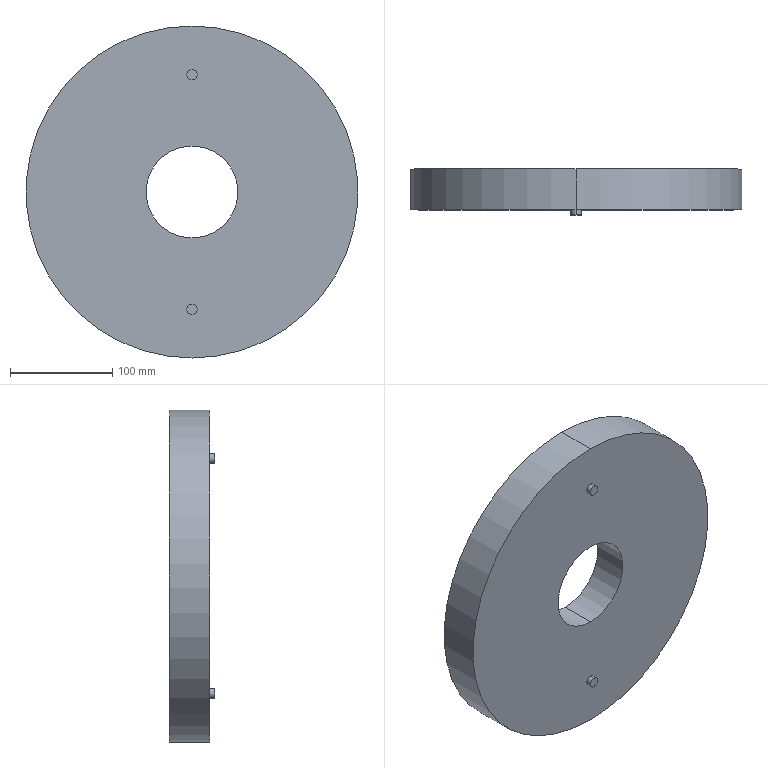Part | SolidWorks | features BaseBody 1 | 1 solid | 15 faces | box 325 x 45 x 325 mm | volume 2743003 mm3 | cylinder 10 | plane 5 | commonest cylinder face diameters 10 x4 90 x2 300 x2 325 x2
STEP:
#1=CARTESIAN_POINT('',(0.,-5.,110.));
#2=VERTEX_POINT('',#1);
#3=CARTESIAN_POINT('',(0.,-5.,120.));
#4=VERTEX_POINT('',#3);
#5=CARTESIAN_POINT('',(0.,-5.,115.));
#6=DIRECTION('',(0.,-1.,0.));
#7=DIRECTION('',(0.,0.,-1.));
#8=AXIS2_PLACEMENT_3D('',#5,#6,#7);
#9=CIRCLE('',#8,5.);
#10=EDGE_CURVE('',#2,#4,#9,.T.);
#11=ORIENTED_EDGE('',*,*,#10,.F.);
#12=CARTESIAN_POINT('',(0.,0.,110.));
#13=VERTEX_POINT('',#12);
#14=CARTESIAN_POINT('',(0.,-5.,110.));
#15=DIRECTION('',(0.,1.,0.));
#16=VECTOR('',#15,1000.);
#17=LINE('',#14,#16);
#18=EDGE_CURVE('',#2,#13,#17,.T.);
#19=ORIENTED_EDGE('',*,*,#18,.T.);
#20=CARTESIAN_POINT('',(0.,0.,120.));
#21=VERTEX_POINT('',#20);
#22=CARTESIAN_POINT('',(0.,0.,115.));
#23=DIRECTION('',(0.,-1.,0.));
#24=DIRECTION('',(0.,0.,1.));
#25=AXIS2_PLACEMENT_3D('',#22,#23,#24);
#26=CIRCLE('',#25,5.);
#27=EDGE_CURVE('',#13,#21,#26,.T.);
#28=ORIENTED_EDGE('',*,*,#27,.T.);
#29=CARTESIAN_POINT('',(0.,-5.,120.));
#30=DIRECTION('',(0.,1.,0.));
#31=VECTOR('',#30,1000.);
#32=LINE('',#29,#31);
#33=EDGE_CURVE('',#4,#21,#32,.T.);
#34=ORIENTED_EDGE('',*,*,#33,.F.);
#35=EDGE_LOOP('',(#11,#19,#28,#34));
#36=FACE_OUTER_BOUND('',#35,.T.);
#37=CARTESIAN_POINT('',(0.,-5.,115.));
#38=DIRECTION('',(0.,1.,0.));
#39=DIRECTION('',(0.,0.,1.));
#40=AXIS2_PLACEMENT_3D('',#37,#38,#39);
#41=CYLINDRICAL_SURFACE('',#40,5.);
#42=ADVANCED_FACE('',(#36),#41,.T.);
#43=CARTESIAN_POINT('',(0.,-5.,-120.));
#44=VERTEX_POINT('',#43);
#45=CARTESIAN_POINT('',(0.,-5.,-110.));
#46=VERTEX_POINT('',#45);
#47=CARTESIAN_POINT('',(0.,-5.,-115.));
#48=DIRECTION('',(0.,-1.,0.));
#49=DIRECTION('',(0.,0.,-1.));
#50=AXIS2_PLACEMENT_3D('',#47,#48,#49);
#51=CIRCLE('',#50,5.);
#52=EDGE_CURVE('',#44,#46,#51,.T.);
#53=ORIENTED_EDGE('',*,*,#52,.F.);
#54=CARTESIAN_POINT('',(0.,0.,-120.));
#55=VERTEX_POINT('',#54);
#56=CARTESIAN_POINT('',(0.,-5.,-120.));
#57=DIRECTION('',(0.,1.,0.));
#58=VECTOR('',#57,1000.);
#59=LINE('',#56,#58);
#60=EDGE_CURVE('',#44,#55,#59,.T.);
#61=ORIENTED_EDGE('',*,*,#60,.T.);
#62=CARTESIAN_POINT('',(0.,0.,-110.));
#63=VERTEX_POINT('',#62);
#64=CARTESIAN_POINT('',(0.,0.,-115.));
#65=DIRECTION('',(0.,-1.,0.));
#66=DIRECTION('',(0.,0.,1.));
#67=AXIS2_PLACEMENT_3D('',#64,#65,#66);
#68=CIRCLE('',#67,5.);
#69=EDGE_CURVE('',#55,#63,#68,.T.);
#70=ORIENTED_EDGE('',*,*,#69,.T.);
#71=CARTESIAN_POINT('',(0.,-5.,-110.));
#72=DIRECTION('',(0.,1.,0.));
#73=VECTOR('',#72,1000.);
#74=LINE('',#71,#73);
#75=EDGE_CURVE('',#46,#63,#74,.T.);
#76=ORIENTED_EDGE('',*,*,#75,.F.);
#77=EDGE_LOOP('',(#53,#61,#70,#76));
#78=FACE_OUTER_BOUND('',#77,.T.);
#79=CARTESIAN_POINT('',(0.,-5.,-115.));
#80=DIRECTION('',(0.,1.,0.));
#81=DIRECTION('',(0.,0.,1.));
#82=AXIS2_PLACEMENT_3D('',#79,#80,#81);
#83=CYLINDRICAL_SURFACE('',#82,5.);
#84=ADVANCED_FACE('',(#78),#83,.T.);
#85=CARTESIAN_POINT('',(0.,0.,-45.));
#86=VERTEX_POINT('',#85);
#87=CARTESIAN_POINT('',(0.,0.,45.));
#88=VERTEX_POINT('',#87);
#89=CARTESIAN_POINT('',(0.,0.,0.));
#90=DIRECTION('',(0.,1.,0.));
#91=DIRECTION('',(0.,0.,1.));
#92=AXIS2_PLACEMENT_3D('',#89,#90,#91);
#93=CIRCLE('',#92,45.);
#94=EDGE_CURVE('',#86,#88,#93,.T.);
#95=ORIENTED_EDGE('',*,*,#94,.F.);
#96=CARTESIAN_POINT('',(0.,35.,-45.));
#97=VERTEX_POINT('',#96);
#98=CARTESIAN_POINT('',(0.,0.,-45.));
#99=DIRECTION('',(0.,1.,0.));
#100=VECTOR('',#99,1000.);
#101=LINE('',#98,#100);
#102=EDGE_CURVE('',#86,#97,#101,.T.);
#103=ORIENTED_EDGE('',*,*,#102,.T.);
#104=CARTESIAN_POINT('',(0.,35.,45.));
#105=VERTEX_POINT('',#104);
#106=CARTESIAN_POINT('',(0.,35.,0.));
#107=DIRECTION('',(0.,1.,0.));
#108=DIRECTION('',(0.,0.,1.));
#109=AXIS2_PLACEMENT_3D('',#106,#107,#108);
#110=CIRCLE('',#109,45.);
#111=EDGE_CURVE('',#97,#105,#110,.T.);
#112=ORIENTED_EDGE('',*,*,#111,.T.);
#113=CARTESIAN_POINT('',(0.,0.,45.));
#114=DIRECTION('',(0.,1.,0.));
#115=VECTOR('',#114,1000.);
#116=LINE('',#113,#115);
#117=EDGE_CURVE('',#88,#105,#116,.T.);
#118=ORIENTED_EDGE('',*,*,#117,.F.);
#119=EDGE_LOOP('',(#95,#103,#112,#118));
#120=FACE_OUTER_BOUND('',#119,.T.);
#121=CARTESIAN_POINT('',(0.,0.,0.));
#122=DIRECTION('',(0.,1.,0.));
#123=DIRECTION('',(0.,0.,1.));
#124=AXIS2_PLACEMENT_3D('',#121,#122,#123);
#125=CYLINDRICAL_SURFACE('',#124,45.);
#126=ADVANCED_FACE('',(#120),#125,.F.);
#127=CARTESIAN_POINT('',(0.,35.,-150.));
#128=VERTEX_POINT('',#127);
#129=CARTESIAN_POINT('',(0.,35.,150.));
#130=VERTEX_POINT('',#129);
#131=CARTESIAN_POINT('',(0.,35.,0.));
#132=DIRECTION('',(0.,1.,0.));
#133=DIRECTION('',(0.,0.,1.));
#134=AXIS2_PLACEMENT_3D('',#131,#132,#133);
#135=CIRCLE('',#134,150.);
#136=EDGE_CURVE('',#128,#130,#135,.T.);
#137=ORIENTED_EDGE('',*,*,#136,.F.);
#138=CARTESIAN_POINT('',(0.,40.,-150.));
#139=VERTEX_POINT('',#138);
#140=CARTESIAN_POINT('',(0.,35.,-150.));
#141=DIRECTION('',(0.,1.,0.));
#142=VECTOR('',#141,1000.);
#143=LINE('',#140,#142);
#144=EDGE_CURVE('',#128,#139,#143,.T.);
#145=ORIENTED_EDGE('',*,*,#144,.T.);
#146=CARTESIAN_POINT('',(0.,40.,150.));
#147=VERTEX_POINT('',#146);
#148=CARTESIAN_POINT('',(0.,40.,0.));
#149=DIRECTION('',(0.,1.,0.));
#150=DIRECTION('',(0.,0.,1.));
#151=AXIS2_PLACEMENT_3D('',#148,#149,#150);
#152=CIRCLE('',#151,150.);
#153=EDGE_CURVE('',#139,#147,#152,.T.);
#154=ORIENTED_EDGE('',*,*,#153,.T.);
#155=CARTESIAN_POINT('',(0.,35.,150.));
#156=DIRECTION('',(0.,1.,0.));
#157=VECTOR('',#156,1000.);
#158=LINE('',#155,#157);
#159=EDGE_CURVE('',#130,#147,#158,.T.);
#160=ORIENTED_EDGE('',*,*,#159,.F.);
#161=EDGE_LOOP('',(#137,#145,#154,#160));
#162=FACE_OUTER_BOUND('',#161,.T.);
#163=CARTESIAN_POINT('',(0.,35.,0.));
#164=DIRECTION('',(0.,1.,0.));
#165=DIRECTION('',(0.,0.,1.));
#166=AXIS2_PLACEMENT_3D('',#163,#164,#165);
#167=CYLINDRICAL_SURFACE('',#166,150.);
#168=ADVANCED_FACE('',(#162),#167,.F.);
#169=CARTESIAN_POINT('',(0.,40.,162.5));
#170=VERTEX_POINT('',#169);
#171=CARTESIAN_POINT('',(0.,40.,-162.5));
#172=VERTEX_POINT('',#171);
#173=CARTESIAN_POINT('',(0.,40.,0.));
#174=DIRECTION('',(0.,1.,0.));
#175=DIRECTION('',(0.,0.,1.));
#176=AXIS2_PLACEMENT_3D('',#173,#174,#175);
#177=CIRCLE('',#176,162.5);
#178=EDGE_CURVE('',#170,#172,#177,.T.);
#179=ORIENTED_EDGE('',*,*,#178,.F.);
#180=CARTESIAN_POINT('',(0.,0.,162.5));
#181=VERTEX_POINT('',#180);
#182=CARTESIAN_POINT('',(0.,40.,162.5));
#183=DIRECTION('',(0.,-1.,0.));
#184=VECTOR('',#183,1000.);
#185=LINE('',#182,#184);
#186=EDGE_CURVE('',#170,#181,#185,.T.);
#187=ORIENTED_EDGE('',*,*,#186,.T.);
#188=CARTESIAN_POINT('',(0.,0.,-162.5));
#189=VERTEX_POINT('',#188);
#190=CARTESIAN_POINT('',(0.,0.,0.));
#191=DIRECTION('',(0.,1.,0.));
#192=DIRECTION('',(0.,0.,1.));
#193=AXIS2_PLACEMENT_3D('',#190,#191,#192);
#194=CIRCLE('',#193,162.5);
#195=EDGE_CURVE('',#181,#189,#194,.T.);
#196=ORIENTED_EDGE('',*,*,#195,.T.);
#197=CARTESIAN_POINT('',(0.,40.,-162.5));
#198=DIRECTION('',(0.,-1.,0.));
#199=VECTOR('',#198,1000.);
#200=LINE('',#197,#199);
#201=EDGE_CURVE('',#172,#189,#200,.T.);
#202=ORIENTED_EDGE('',*,*,#201,.F.);
#203=EDGE_LOOP('',(#179,#187,#196,#202));
#204=FACE_OUTER_BOUND('',#203,.T.);
#205=CARTESIAN_POINT('',(0.,40.,0.));
#206=DIRECTION('',(0.,-1.,0.));
#207=DIRECTION('',(0.,0.,-1.));
#208=AXIS2_PLACEMENT_3D('',#205,#206,#207);
#209=CYLINDRICAL_SURFACE('',#208,162.5);
#210=ADVANCED_FACE('',(#204),#209,.T.);
#211=ORIENTED_EDGE('',*,*,#186,.F.);
#212=CARTESIAN_POINT('',(0.,40.,0.));
#213=DIRECTION('',(0.,1.,0.));
#214=DIRECTION('',(0.,0.,1.));
#215=AXIS2_PLACEMENT_3D('',#212,#213,#214);
#216=CIRCLE('',#215,162.5);
#217=EDGE_CURVE('',#172,#170,#216,.T.);
#218=ORIENTED_EDGE('',*,*,#217,.F.);
#219=ORIENTED_EDGE('',*,*,#201,.T.);
#220=CARTESIAN_POINT('',(0.,0.,0.));
#221=DIRECTION('',(0.,1.,0.));
#222=DIRECTION('',(0.,0.,1.));
#223=AXIS2_PLACEMENT_3D('',#220,#221,#222);
#224=CIRCLE('',#223,162.5);
#225=EDGE_CURVE('',#189,#181,#224,.T.);
#226=ORIENTED_EDGE('',*,*,#225,.T.);
#227=EDGE_LOOP('',(#211,#218,#219,#226));
#228=FACE_OUTER_BOUND('',#227,.T.);
#229=CARTESIAN_POINT('',(0.,40.,0.));
#230=DIRECTION('',(0.,-1.,0.));
#231=DIRECTION('',(0.,0.,-1.));
#232=AXIS2_PLACEMENT_3D('',#229,#230,#231);
#233=CYLINDRICAL_SURFACE('',#232,162.5);
#234=ADVANCED_FACE('',(#228),#233,.T.);
#235=CARTESIAN_POINT('',(0.,40.,0.));
#236=DIRECTION('',(0.,1.,0.));
#237=DIRECTION('',(0.,0.,1.));
#238=AXIS2_PLACEMENT_3D('',#235,#236,#237);
#239=CIRCLE('',#238,150.);
#240=EDGE_CURVE('',#147,#139,#239,.T.);
#241=ORIENTED_EDGE('',*,*,#240,.F.);
#242=ORIENTED_EDGE('',*,*,#153,.F.);
#243=EDGE_LOOP('',(#241,#242));
#244=FACE_BOUND('',#243,.T.);
#245=ORIENTED_EDGE('',*,*,#217,.T.);
#246=ORIENTED_EDGE('',*,*,#178,.T.);
#247=EDGE_LOOP('',(#245,#246));
#248=FACE_OUTER_BOUND('',#247,.T.);
#249=CARTESIAN_POINT('',(0.,40.,0.));
#250=DIRECTION('',(0.,1.,0.));
#251=DIRECTION('',(0.,0.,1.));
#252=AXIS2_PLACEMENT_3D('',#249,#250,#251);
#253=PLANE('',#252);
#254=ADVANCED_FACE('',(#244,#248),#253,.T.);
#255=CARTESIAN_POINT('',(0.,0.,115.));
#256=DIRECTION('',(0.,-1.,0.));
#257=DIRECTION('',(0.,0.,1.));
#258=AXIS2_PLACEMENT_3D('',#255,#256,#257);
#259=CIRCLE('',#258,5.);
#260=EDGE_CURVE('',#21,#13,#259,.T.);
#261=ORIENTED_EDGE('',*,*,#260,.F.);
#262=ORIENTED_EDGE('',*,*,#27,.F.);
#263=EDGE_LOOP('',(#261,#262));
#264=FACE_BOUND('',#263,.T.);
#265=CARTESIAN_POINT('',(0.,0.,-115.));
#266=DIRECTION('',(0.,-1.,0.));
#267=DIRECTION('',(0.,0.,1.));
#268=AXIS2_PLACEMENT_3D('',#265,#266,#267);
#269=CIRCLE('',#268,5.);
#270=EDGE_CURVE('',#63,#55,#269,.T.);
#271=ORIENTED_EDGE('',*,*,#270,.F.);
#272=ORIENTED_EDGE('',*,*,#69,.F.);
#273=EDGE_LOOP('',(#271,#272));
#274=FACE_BOUND('',#273,.T.);
#275=CARTESIAN_POINT('',(0.,0.,0.));
#276=DIRECTION('',(0.,1.,0.));
#277=DIRECTION('',(0.,0.,1.));
#278=AXIS2_PLACEMENT_3D('',#275,#276,#277);
#279=CIRCLE('',#278,45.);
#280=EDGE_CURVE('',#88,#86,#279,.T.);
#281=ORIENTED_EDGE('',*,*,#280,.T.);
#282=ORIENTED_EDGE('',*,*,#94,.T.);
#283=EDGE_LOOP('',(#281,#282));
#284=FACE_BOUND('',#283,.T.);
#285=ORIENTED_EDGE('',*,*,#225,.F.);
#286=ORIENTED_EDGE('',*,*,#195,.F.);
#287=EDGE_LOOP('',(#285,#286));
#288=FACE_OUTER_BOUND('',#287,.T.);
#289=CARTESIAN_POINT('',(0.,0.,0.));
#290=DIRECTION('',(0.,1.,0.));
#291=DIRECTION('',(0.,0.,1.));
#292=AXIS2_PLACEMENT_3D('',#289,#290,#291);
#293=PLANE('',#292);
#294=ADVANCED_FACE('',(#264,#274,#284,#288),#293,.F.);
#295=ORIENTED_EDGE('',*,*,#144,.F.);
#296=CARTESIAN_POINT('',(0.,35.,0.));
#297=DIRECTION('',(0.,1.,0.));
#298=DIRECTION('',(0.,0.,1.));
#299=AXIS2_PLACEMENT_3D('',#296,#297,#298);
#300=CIRCLE('',#299,150.);
#301=EDGE_CURVE('',#130,#128,#300,.T.);
#302=ORIENTED_EDGE('',*,*,#301,.F.);
#303=ORIENTED_EDGE('',*,*,#159,.T.);
#304=ORIENTED_EDGE('',*,*,#240,.T.);
#305=EDGE_LOOP('',(#295,#302,#303,#304));
#306=FACE_OUTER_BOUND('',#305,.T.);
#307=CARTESIAN_POINT('',(0.,35.,0.));
#308=DIRECTION('',(0.,1.,0.));
#309=DIRECTION('',(0.,0.,1.));
#310=AXIS2_PLACEMENT_3D('',#307,#308,#309);
#311=CYLINDRICAL_SURFACE('',#310,150.);
#312=ADVANCED_FACE('',(#306),#311,.F.);
#313=CARTESIAN_POINT('',(0.,35.,0.));
#314=DIRECTION('',(0.,1.,0.));
#315=DIRECTION('',(0.,0.,1.));
#316=AXIS2_PLACEMENT_3D('',#313,#314,#315);
#317=CIRCLE('',#316,45.);
#318=EDGE_CURVE('',#105,#97,#317,.T.);
#319=ORIENTED_EDGE('',*,*,#318,.F.);
#320=ORIENTED_EDGE('',*,*,#111,.F.);
#321=EDGE_LOOP('',(#319,#320));
#322=FACE_BOUND('',#321,.T.);
#323=ORIENTED_EDGE('',*,*,#301,.T.);
#324=ORIENTED_EDGE('',*,*,#136,.T.);
#325=EDGE_LOOP('',(#323,#324));
#326=FACE_OUTER_BOUND('',#325,.T.);
#327=CARTESIAN_POINT('',(0.,35.,0.));
#328=DIRECTION('',(0.,1.,0.));
#329=DIRECTION('',(0.,0.,1.));
#330=AXIS2_PLACEMENT_3D('',#327,#328,#329);
#331=PLANE('',#330);
#332=ADVANCED_FACE('',(#322,#326),#331,.T.);
#333=ORIENTED_EDGE('',*,*,#102,.F.);
#334=ORIENTED_EDGE('',*,*,#280,.F.);
#335=ORIENTED_EDGE('',*,*,#117,.T.);
#336=ORIENTED_EDGE('',*,*,#318,.T.);
#337=EDGE_LOOP('',(#333,#334,#335,#336));
#338=FACE_OUTER_BOUND('',#337,.T.);
#339=CARTESIAN_POINT('',(0.,0.,0.));
#340=DIRECTION('',(0.,1.,0.));
#341=DIRECTION('',(0.,0.,1.));
#342=AXIS2_PLACEMENT_3D('',#339,#340,#341);
#343=CYLINDRICAL_SURFACE('',#342,45.);
#344=ADVANCED_FACE('',(#338),#343,.F.);
#345=ORIENTED_EDGE('',*,*,#60,.F.);
#346=CARTESIAN_POINT('',(0.,-5.,-115.));
#347=DIRECTION('',(0.,-1.,0.));
#348=DIRECTION('',(0.,0.,-1.));
#349=AXIS2_PLACEMENT_3D('',#346,#347,#348);
#350=CIRCLE('',#349,5.);
#351=EDGE_CURVE('',#46,#44,#350,.T.);
#352=ORIENTED_EDGE('',*,*,#351,.F.);
#353=ORIENTED_EDGE('',*,*,#75,.T.);
#354=ORIENTED_EDGE('',*,*,#270,.T.);
#355=EDGE_LOOP('',(#345,#352,#353,#354));
#356=FACE_OUTER_BOUND('',#355,.T.);
#357=CARTESIAN_POINT('',(0.,-5.,-115.));
#358=DIRECTION('',(0.,1.,0.));
#359=DIRECTION('',(0.,0.,1.));
#360=AXIS2_PLACEMENT_3D('',#357,#358,#359);
#361=CYLINDRICAL_SURFACE('',#360,5.);
#362=ADVANCED_FACE('',(#356),#361,.T.);
#363=ORIENTED_EDGE('',*,*,#351,.T.);
#364=ORIENTED_EDGE('',*,*,#52,.T.);
#365=EDGE_LOOP('',(#363,#364));
#366=FACE_OUTER_BOUND('',#365,.T.);
#367=CARTESIAN_POINT('',(0.,-5.,-115.));
#368=DIRECTION('',(0.,-1.,0.));
#369=DIRECTION('',(0.,0.,-1.));
#370=AXIS2_PLACEMENT_3D('',#367,#368,#369);
#371=PLANE('',#370);
#372=ADVANCED_FACE('',(#366),#371,.T.);
#373=ORIENTED_EDGE('',*,*,#18,.F.);
#374=CARTESIAN_POINT('',(0.,-5.,115.));
#375=DIRECTION('',(0.,-1.,0.));
#376=DIRECTION('',(0.,0.,-1.));
#377=AXIS2_PLACEMENT_3D('',#374,#375,#376);
#378=CIRCLE('',#377,5.);
#379=EDGE_CURVE('',#4,#2,#378,.T.);
#380=ORIENTED_EDGE('',*,*,#379,.F.);
#381=ORIENTED_EDGE('',*,*,#33,.T.);
#382=ORIENTED_EDGE('',*,*,#260,.T.);
#383=EDGE_LOOP('',(#373,#380,#381,#382));
#384=FACE_OUTER_BOUND('',#383,.T.);
#385=CARTESIAN_POINT('',(0.,-5.,115.));
#386=DIRECTION('',(0.,1.,0.));
#387=DIRECTION('',(0.,0.,1.));
#388=AXIS2_PLACEMENT_3D('',#385,#386,#387);
#389=CYLINDRICAL_SURFACE('',#388,5.);
#390=ADVANCED_FACE('',(#384),#389,.T.);
#391=ORIENTED_EDGE('',*,*,#379,.T.);
#392=ORIENTED_EDGE('',*,*,#10,.T.);
#393=EDGE_LOOP('',(#391,#392));
#394=FACE_OUTER_BOUND('',#393,.T.);
#395=CARTESIAN_POINT('',(0.,-5.,115.));
#396=DIRECTION('',(0.,-1.,0.));
#397=DIRECTION('',(0.,0.,-1.));
#398=AXIS2_PLACEMENT_3D('',#395,#396,#397);
#399=PLANE('',#398);
#400=ADVANCED_FACE('',(#394),#399,.T.);
#401=CLOSED_SHELL('',(#42,#84,#126,#168,#210,#234,#254,#294,#312,#332,#344,#362,#372,#390,#400));
#402=MANIFOLD_SOLID_BREP('',#401);
#403=CARTESIAN_POINT('',(0.,0.,0.));
#404=DIRECTION('',(0.,0.,1.));
#405=DIRECTION('',(1.,0.,0.));
#406=AXIS2_PLACEMENT_3D('',#403,#404,#405);
#407=(LENGTH_UNIT()NAMED_UNIT(*)SI_UNIT(.MILLI.,.METRE.));
#408=UNCERTAINTY_MEASURE_WITH_UNIT(LENGTH_MEASURE(0.00001),#407,'','');
#409=(NAMED_UNIT(*)PLANE_ANGLE_UNIT()SI_UNIT($,.RADIAN.));
#410=(NAMED_UNIT(*)SI_UNIT($,.STERADIAN.)SOLID_ANGLE_UNIT());
#411=(GEOMETRIC_REPRESENTATION_CONTEXT(3)GLOBAL_UNCERTAINTY_ASSIGNED_CONTEXT((#408))GLOBAL_UNIT_ASSIGNED_CONTEXT((#407,#409,#410))REPRESENTATION_CONTEXT('',''));
#412=ADVANCED_BREP_SHAPE_REPRESENTATION('',(#402,#406),#411);